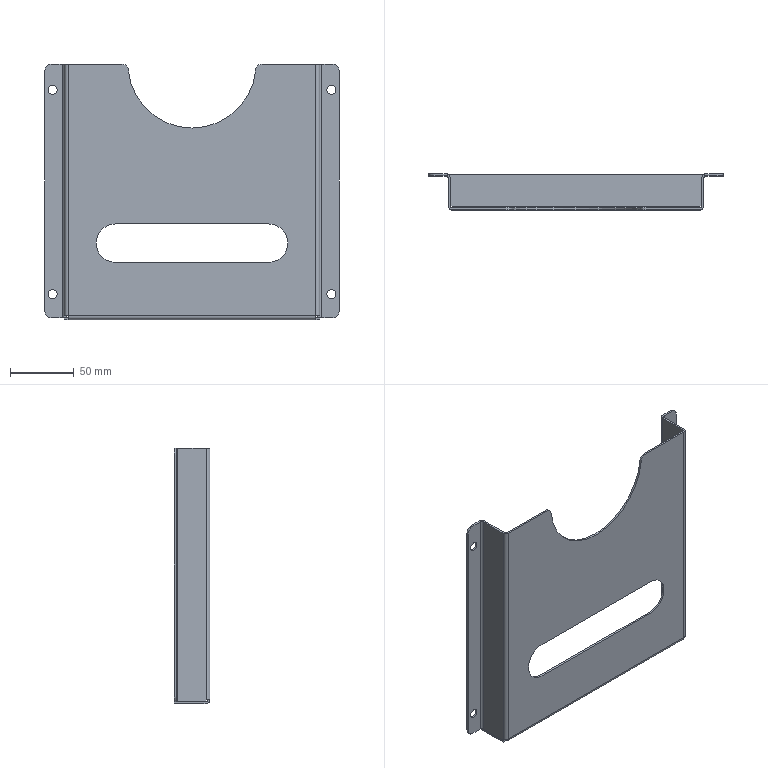Part | NX | features solid 2 | 1 solid | 59 faces | box 230 x 28 x 200 mm | volume 78561 mm3 | plane 31 | cylinder 28 | commonest cylinder face diameters 7 x8 10 x6 3 x5 6 x5 30 x2 100 x2